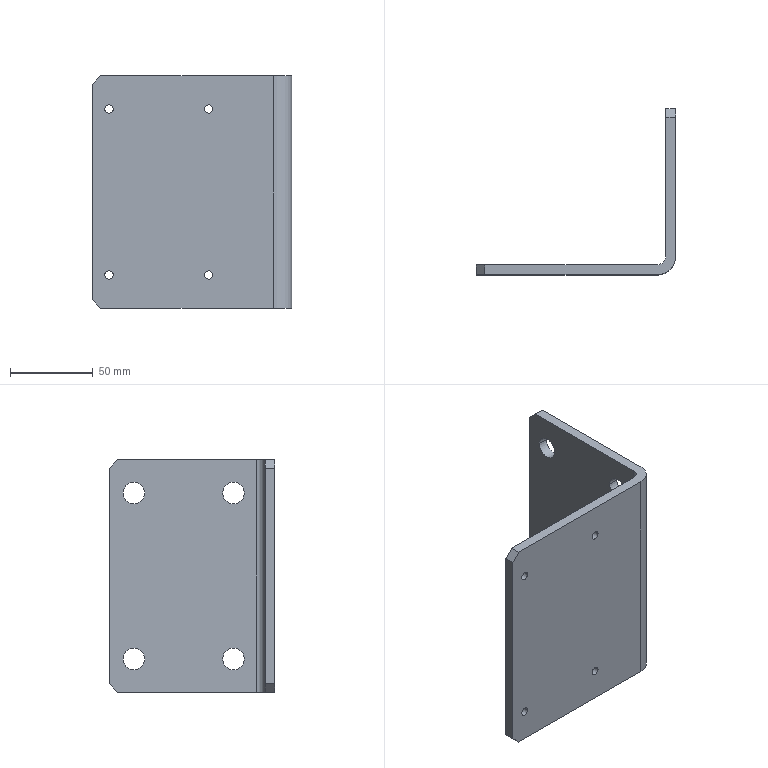Part | STEP file | 1 solid | 30 faces | box 120 x 100 x 140 mm | volume 172919 mm3 | cylinder 18 | plane 12 | commonest cylinder face diameters 5 x8 13 x8 10 x1 22 x1